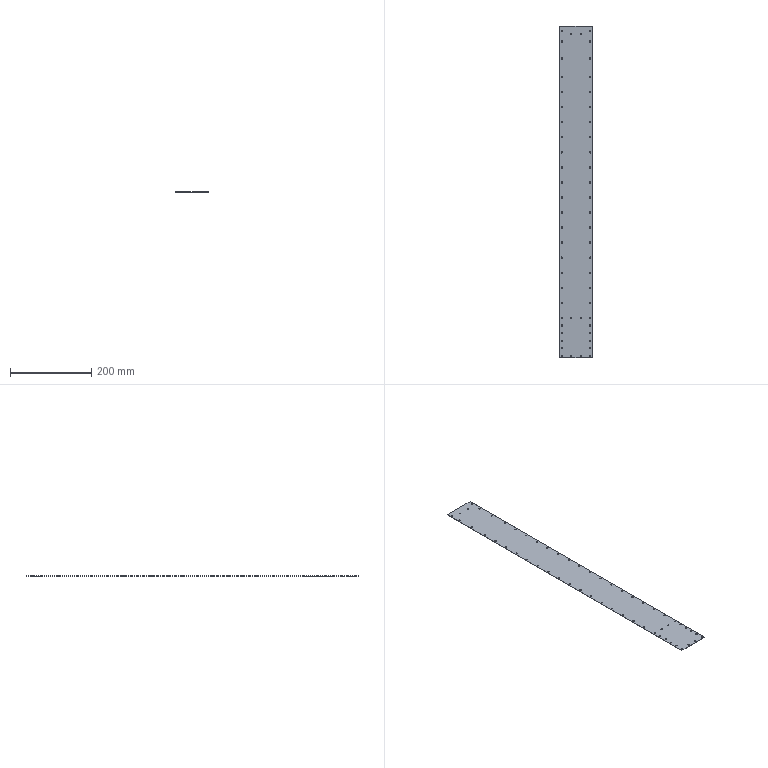Part | SolidWorks | features BaseBody 1 | 1 solid | 118 faces | box 80 x 817 x 0.5 mm | volume 32455 mm3 | cylinder 108 | plane 6 | spline 4 | commonest cylinder face diameters 3.2 x108